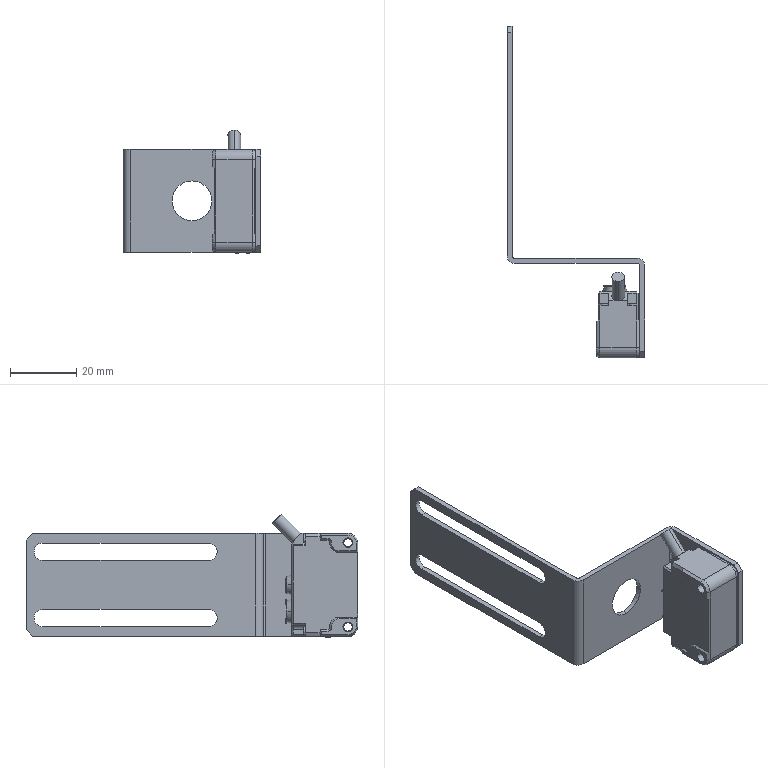Part | SolidWorks | 2 solids | 285 faces | box 41.5 x 100 x 37.32 mm | volume 12746 mm3 | plane 153 | cylinder 115 | cone 17 | commonest cylinder face diameters 0.3 x25 0.5 x22 2.5 x10 3.78 x7 5.2 x6 6 x6